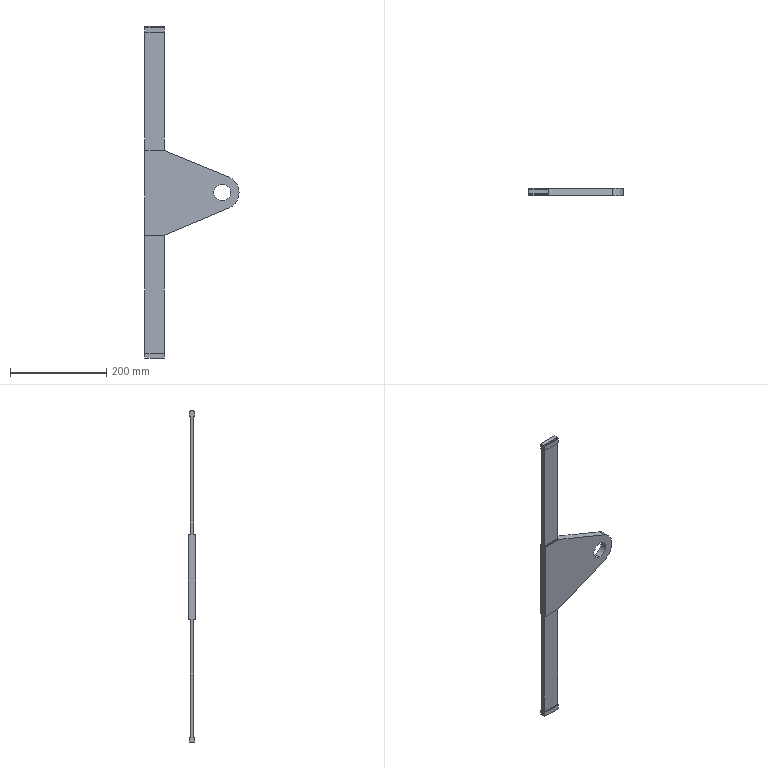Part | SolidWorks | features ICE 6, Cut 1, Extrusion 1, Fillet 1, MirrorPattern 1 | 1 solid | 36 faces | box 195.363 x 15 x 689 mm | volume 515152 mm3 | plane 29 | cylinder 7 | commonest cylinder face diameters 2 x4 35 x2 70 x1
STEP:
#1=CARTESIAN_POINT('',(140.363,7.5,18.413));
#2=VERTEX_POINT('',#1);
#3=CARTESIAN_POINT('',(140.363,7.5,-16.587));
#4=VERTEX_POINT('',#3);
#5=CARTESIAN_POINT('',(140.363,7.5,0.9129));
#6=DIRECTION('',(0.,-1.,0.));
#7=DIRECTION('',(0.,0.,-1.));
#8=AXIS2_PLACEMENT_3D('',#5,#6,#7);
#9=CIRCLE('',#8,17.5);
#10=EDGE_CURVE('',#2,#4,#9,.T.);
#11=ORIENTED_EDGE('',*,*,#10,.F.);
#12=CARTESIAN_POINT('',(140.363,-7.5,18.413));
#13=VERTEX_POINT('',#12);
#14=CARTESIAN_POINT('',(140.363,7.5,18.413));
#15=DIRECTION('',(0.,-1.,0.));
#16=VECTOR('',#15,1000.);
#17=LINE('',#14,#16);
#18=EDGE_CURVE('',#2,#13,#17,.T.);
#19=ORIENTED_EDGE('',*,*,#18,.T.);
#20=CARTESIAN_POINT('',(140.363,-7.5,-16.587));
#21=VERTEX_POINT('',#20);
#22=CARTESIAN_POINT('',(140.363,-7.5,0.9129));
#23=DIRECTION('',(0.,-1.,0.));
#24=DIRECTION('',(0.,0.,-1.));
#25=AXIS2_PLACEMENT_3D('',#22,#23,#24);
#26=CIRCLE('',#25,17.5);
#27=EDGE_CURVE('',#13,#21,#26,.T.);
#28=ORIENTED_EDGE('',*,*,#27,.T.);
#29=CARTESIAN_POINT('',(140.363,7.5,-16.587));
#30=DIRECTION('',(0.,-1.,0.));
#31=VECTOR('',#30,1000.);
#32=LINE('',#29,#31);
#33=EDGE_CURVE('',#4,#21,#32,.T.);
#34=ORIENTED_EDGE('',*,*,#33,.F.);
#35=EDGE_LOOP('',(#11,#19,#28,#34));
#36=FACE_OUTER_BOUND('',#35,.T.);
#37=CARTESIAN_POINT('',(140.363,7.5,0.9129));
#38=DIRECTION('',(0.,-1.,0.));
#39=DIRECTION('',(0.,0.,-1.));
#40=AXIS2_PLACEMENT_3D('',#37,#38,#39);
#41=CYLINDRICAL_SURFACE('',#40,17.5);
#42=ADVANCED_FACE('',(#36),#41,.F.);
#43=CARTESIAN_POINT('',(20.,-4.,-89.));
#44=VERTEX_POINT('',#43);
#45=CARTESIAN_POINT('',(20.,-4.,-332.5));
#46=VERTEX_POINT('',#45);
#47=CARTESIAN_POINT('',(20.,-4.,330.5));
#48=DIRECTION('',(0.,0.,-1.));
#49=VECTOR('',#48,1000.);
#50=LINE('',#47,#49);
#51=EDGE_CURVE('',#44,#46,#50,.T.);
#52=ORIENTED_EDGE('',*,*,#51,.T.);
#53=CARTESIAN_POINT('',(20.,-6.,-332.5));
#54=VERTEX_POINT('',#53);
#55=CARTESIAN_POINT('',(20.,4.,-332.5));
#56=DIRECTION('',(0.,-1.,0.));
#57=VECTOR('',#56,1000.);
#58=LINE('',#55,#57);
#59=EDGE_CURVE('',#46,#54,#58,.T.);
#60=ORIENTED_EDGE('',*,*,#59,.T.);
#61=CARTESIAN_POINT('',(20.,-6.,-342.5));
#62=VERTEX_POINT('',#61);
#63=CARTESIAN_POINT('',(20.,-6.,-333.5));
#64=DIRECTION('',(0.,0.,1.));
#65=VECTOR('',#64,1000.);
#66=LINE('',#63,#65);
#67=EDGE_CURVE('',#62,#54,#66,.T.);
#68=ORIENTED_EDGE('',*,*,#67,.F.);
#69=CARTESIAN_POINT('',(20.,6.,-342.5));
#70=VERTEX_POINT('',#69);
#71=CARTESIAN_POINT('',(20.,-4.,-342.5));
#72=DIRECTION('',(0.,-1.,0.));
#73=VECTOR('',#72,1000.);
#74=LINE('',#71,#73);
#75=EDGE_CURVE('',#70,#62,#74,.T.);
#76=ORIENTED_EDGE('',*,*,#75,.F.);
#77=CARTESIAN_POINT('',(20.,6.,-332.5));
#78=VERTEX_POINT('',#77);
#79=CARTESIAN_POINT('',(20.,6.,-333.5));
#80=DIRECTION('',(0.,0.,-1.));
#81=VECTOR('',#80,1000.);
#82=LINE('',#79,#81);
#83=EDGE_CURVE('',#78,#70,#82,.T.);
#84=ORIENTED_EDGE('',*,*,#83,.F.);
#85=CARTESIAN_POINT('',(20.,4.,-332.5));
#86=VERTEX_POINT('',#85);
#87=CARTESIAN_POINT('',(20.,4.,-332.5));
#88=DIRECTION('',(0.,-1.,0.));
#89=VECTOR('',#88,1000.);
#90=LINE('',#87,#89);
#91=EDGE_CURVE('',#78,#86,#90,.T.);
#92=ORIENTED_EDGE('',*,*,#91,.T.);
#93=CARTESIAN_POINT('',(20.,4.,-89.));
#94=VERTEX_POINT('',#93);
#95=CARTESIAN_POINT('',(20.,4.,330.5));
#96=DIRECTION('',(0.,0.,-1.));
#97=VECTOR('',#96,1000.);
#98=LINE('',#95,#97);
#99=EDGE_CURVE('',#94,#86,#98,.T.);
#100=ORIENTED_EDGE('',*,*,#99,.F.);
#101=CARTESIAN_POINT('',(20.,5.,-88.));
#102=VERTEX_POINT('',#101);
#103=CARTESIAN_POINT('',(20.,5.,-89.));
#104=DIRECTION('',(-1.,0.,0.));
#105=DIRECTION('',(0.,0.,1.));
#106=AXIS2_PLACEMENT_3D('',#103,#104,#105);
#107=CIRCLE('',#106,1.);
#108=EDGE_CURVE('',#94,#102,#107,.T.);
#109=ORIENTED_EDGE('',*,*,#108,.T.);
#110=CARTESIAN_POINT('',(20.,-5.,-88.));
#111=VERTEX_POINT('',#110);
#112=CARTESIAN_POINT('',(20.,-7.5,-88.));
#113=DIRECTION('',(0.,1.,0.));
#114=VECTOR('',#113,1000.);
#115=LINE('',#112,#114);
#116=EDGE_CURVE('',#111,#102,#115,.T.);
#117=ORIENTED_EDGE('',*,*,#116,.F.);
#118=CARTESIAN_POINT('',(20.,-5.,-89.));
#119=DIRECTION('',(-1.,0.,0.));
#120=DIRECTION('',(0.,0.,1.));
#121=AXIS2_PLACEMENT_3D('',#118,#119,#120);
#122=CIRCLE('',#121,1.);
#123=EDGE_CURVE('',#111,#44,#122,.T.);
#124=ORIENTED_EDGE('',*,*,#123,.T.);
#125=EDGE_LOOP('',(#52,#60,#68,#76,#84,#92,#100,#109,#117,#124));
#126=FACE_OUTER_BOUND('',#125,.T.);
#127=CARTESIAN_POINT('',(20.,-4.,330.5));
#128=DIRECTION('',(-1.,0.,0.));
#129=DIRECTION('',(0.,0.,1.));
#130=AXIS2_PLACEMENT_3D('',#127,#128,#129);
#131=PLANE('',#130);
#132=ADVANCED_FACE('',(#126),#131,.F.);
#133=CARTESIAN_POINT('',(-20.,4.,-89.));
#134=VERTEX_POINT('',#133);
#135=CARTESIAN_POINT('',(-20.,4.,-332.5));
#136=VERTEX_POINT('',#135);
#137=CARTESIAN_POINT('',(-20.,4.,330.5));
#138=DIRECTION('',(0.,0.,-1.));
#139=VECTOR('',#138,1000.);
#140=LINE('',#137,#139);
#141=EDGE_CURVE('',#134,#136,#140,.T.);
#142=ORIENTED_EDGE('',*,*,#141,.T.);
#143=CARTESIAN_POINT('',(-20.,6.,-332.5));
#144=VERTEX_POINT('',#143);
#145=CARTESIAN_POINT('',(-20.,4.,-332.5));
#146=DIRECTION('',(0.,1.,0.));
#147=VECTOR('',#146,1000.);
#148=LINE('',#145,#147);
#149=EDGE_CURVE('',#136,#144,#148,.T.);
#150=ORIENTED_EDGE('',*,*,#149,.T.);
#151=CARTESIAN_POINT('',(-20.,6.,-342.5));
#152=VERTEX_POINT('',#151);
#153=CARTESIAN_POINT('',(-20.,6.,-333.5));
#154=DIRECTION('',(0.,0.,1.));
#155=VECTOR('',#154,1000.);
#156=LINE('',#153,#155);
#157=EDGE_CURVE('',#152,#144,#156,.T.);
#158=ORIENTED_EDGE('',*,*,#157,.F.);
#159=CARTESIAN_POINT('',(-20.,-6.,-342.5));
#160=VERTEX_POINT('',#159);
#161=CARTESIAN_POINT('',(-20.,-4.,-342.5));
#162=DIRECTION('',(0.,1.,0.));
#163=VECTOR('',#162,1000.);
#164=LINE('',#161,#163);
#165=EDGE_CURVE('',#160,#152,#164,.T.);
#166=ORIENTED_EDGE('',*,*,#165,.F.);
#167=CARTESIAN_POINT('',(-20.,-6.,-332.5));
#168=VERTEX_POINT('',#167);
#169=CARTESIAN_POINT('',(-20.,-6.,-333.5));
#170=DIRECTION('',(0.,0.,-1.));
#171=VECTOR('',#170,1000.);
#172=LINE('',#169,#171);
#173=EDGE_CURVE('',#168,#160,#172,.T.);
#174=ORIENTED_EDGE('',*,*,#173,.F.);
#175=CARTESIAN_POINT('',(-20.,-4.,-332.5));
#176=VERTEX_POINT('',#175);
#177=CARTESIAN_POINT('',(-20.,4.,-332.5));
#178=DIRECTION('',(0.,1.,0.));
#179=VECTOR('',#178,1000.);
#180=LINE('',#177,#179);
#181=EDGE_CURVE('',#168,#176,#180,.T.);
#182=ORIENTED_EDGE('',*,*,#181,.T.);
#183=CARTESIAN_POINT('',(-20.,-4.,-89.));
#184=VERTEX_POINT('',#183);
#185=CARTESIAN_POINT('',(-20.,-4.,330.5));
#186=DIRECTION('',(0.,0.,-1.));
#187=VECTOR('',#186,1000.);
#188=LINE('',#185,#187);
#189=EDGE_CURVE('',#184,#176,#188,.T.);
#190=ORIENTED_EDGE('',*,*,#189,.F.);
#191=CARTESIAN_POINT('',(-20.,-5.,-88.));
#192=VERTEX_POINT('',#191);
#193=CARTESIAN_POINT('',(-20.,-5.,-89.));
#194=DIRECTION('',(1.,0.,0.));
#195=DIRECTION('',(0.,0.,-1.));
#196=AXIS2_PLACEMENT_3D('',#193,#194,#195);
#197=CIRCLE('',#196,1.);
#198=EDGE_CURVE('',#184,#192,#197,.T.);
#199=ORIENTED_EDGE('',*,*,#198,.T.);
#200=CARTESIAN_POINT('',(-20.,-7.5,-88.));
#201=VERTEX_POINT('',#200);
#202=CARTESIAN_POINT('',(-20.,-4.,-88.));
#203=DIRECTION('',(0.,1.,0.));
#204=VECTOR('',#203,1000.);
#205=LINE('',#202,#204);
#206=EDGE_CURVE('',#201,#192,#205,.T.);
#207=ORIENTED_EDGE('',*,*,#206,.F.);
#208=CARTESIAN_POINT('',(-20.,-7.5,88.));
#209=VERTEX_POINT('',#208);
#210=CARTESIAN_POINT('',(-20.,-7.5,-88.));
#211=DIRECTION('',(0.,0.,-1.));
#212=VECTOR('',#211,1000.);
#213=LINE('',#210,#212);
#214=EDGE_CURVE('',#209,#201,#213,.T.);
#215=ORIENTED_EDGE('',*,*,#214,.F.);
#216=CARTESIAN_POINT('',(-20.,-5.,88.));
#217=VERTEX_POINT('',#216);
#218=CARTESIAN_POINT('',(-20.,-7.5,88.));
#219=DIRECTION('',(0.,-1.,0.));
#220=VECTOR('',#219,1000.);
#221=LINE('',#218,#220);
#222=EDGE_CURVE('',#217,#209,#221,.T.);
#223=ORIENTED_EDGE('',*,*,#222,.F.);
#224=CARTESIAN_POINT('',(-20.,-4.,89.));
#225=VERTEX_POINT('',#224);
#226=CARTESIAN_POINT('',(-20.,-5.,89.));
#227=DIRECTION('',(1.,0.,0.));
#228=DIRECTION('',(0.,0.,-1.));
#229=AXIS2_PLACEMENT_3D('',#226,#227,#228);
#230=CIRCLE('',#229,1.);
#231=EDGE_CURVE('',#217,#225,#230,.T.);
#232=ORIENTED_EDGE('',*,*,#231,.T.);
#233=CARTESIAN_POINT('',(-20.,-4.,333.5));
#234=VERTEX_POINT('',#233);
#235=CARTESIAN_POINT('',(-20.,-4.,330.5));
#236=DIRECTION('',(0.,0.,-1.));
#237=VECTOR('',#236,1000.);
#238=LINE('',#235,#237);
#239=EDGE_CURVE('',#234,#225,#238,.T.);
#240=ORIENTED_EDGE('',*,*,#239,.F.);
#241=CARTESIAN_POINT('',(-20.,-6.,333.5));
#242=VERTEX_POINT('',#241);
#243=CARTESIAN_POINT('',(-20.,-6.,333.5));
#244=DIRECTION('',(0.,-1.,0.));
#245=VECTOR('',#244,1000.);
#246=LINE('',#243,#245);
#247=EDGE_CURVE('',#234,#242,#246,.T.);
#248=ORIENTED_EDGE('',*,*,#247,.T.);
#249=CARTESIAN_POINT('',(-20.,-6.,343.5));
#250=VERTEX_POINT('',#249);
#251=CARTESIAN_POINT('',(-20.,-6.,333.5));
#252=DIRECTION('',(0.,0.,1.));
#253=VECTOR('',#252,1000.);
#254=LINE('',#251,#253);
#255=EDGE_CURVE('',#242,#250,#254,.T.);
#256=ORIENTED_EDGE('',*,*,#255,.T.);
#257=CARTESIAN_POINT('',(-20.,-4.,343.5));
#258=VERTEX_POINT('',#257);
#259=CARTESIAN_POINT('',(-20.,-6.,343.5));
#260=DIRECTION('',(0.,1.,0.));
#261=VECTOR('',#260,1000.);
#262=LINE('',#259,#261);
#263=EDGE_CURVE('',#250,#258,#262,.T.);
#264=ORIENTED_EDGE('',*,*,#263,.T.);
#265=CARTESIAN_POINT('',(-20.,-4.,346.5));
#266=VERTEX_POINT('',#265);
#267=CARTESIAN_POINT('',(-20.,-4.,343.5));
#268=DIRECTION('',(0.,0.,1.));
#269=VECTOR('',#268,1000.);
#270=LINE('',#267,#269);
#271=EDGE_CURVE('',#258,#266,#270,.T.);
#272=ORIENTED_EDGE('',*,*,#271,.T.);
#273=CARTESIAN_POINT('',(-20.,4.,346.5));
#274=VERTEX_POINT('',#273);
#275=CARTESIAN_POINT('',(-20.,0.5169,346.5));
#276=DIRECTION('',(0.,1.,0.));
#277=VECTOR('',#276,1000.);
#278=LINE('',#275,#277);
#279=EDGE_CURVE('',#266,#274,#278,.T.);
#280=ORIENTED_EDGE('',*,*,#279,.T.);
#281=CARTESIAN_POINT('',(-20.,4.,343.5));
#282=VERTEX_POINT('',#281);
#283=CARTESIAN_POINT('',(-20.,4.,343.5));
#284=DIRECTION('',(0.,0.,-1.));
#285=VECTOR('',#284,1000.);
#286=LINE('',#283,#285);
#287=EDGE_CURVE('',#274,#282,#286,.T.);
#288=ORIENTED_EDGE('',*,*,#287,.T.);
#289=CARTESIAN_POINT('',(-20.,6.,343.5));
#290=VERTEX_POINT('',#289);
#291=CARTESIAN_POINT('',(-20.,4.,343.5));
#292=DIRECTION('',(0.,1.,0.));
#293=VECTOR('',#292,1000.);
#294=LINE('',#291,#293);
#295=EDGE_CURVE('',#282,#290,#294,.T.);
#296=ORIENTED_EDGE('',*,*,#295,.T.);
#297=CARTESIAN_POINT('',(-20.,6.,333.5));
#298=VERTEX_POINT('',#297);
#299=CARTESIAN_POINT('',(-20.,6.,333.5));
#300=DIRECTION('',(0.,0.,-1.));
#301=VECTOR('',#300,1000.);
#302=LINE('',#299,#301);
#303=EDGE_CURVE('',#290,#298,#302,.T.);
#304=ORIENTED_EDGE('',*,*,#303,.T.);
#305=CARTESIAN_POINT('',(-20.,4.,333.5));
#306=VERTEX_POINT('',#305);
#307=CARTESIAN_POINT('',(-20.,4.,333.5));
#308=DIRECTION('',(0.,-1.,0.));
#309=VECTOR('',#308,1000.);
#310=LINE('',#307,#309);
#311=EDGE_CURVE('',#298,#306,#310,.T.);
#312=ORIENTED_EDGE('',*,*,#311,.T.);
#313=CARTESIAN_POINT('',(-20.,4.,89.));
#314=VERTEX_POINT('',#313);
#315=CARTESIAN_POINT('',(-20.,4.,330.5));
#316=DIRECTION('',(0.,0.,-1.));
#317=VECTOR('',#316,1000.);
#318=LINE('',#315,#317);
#319=EDGE_CURVE('',#306,#314,#318,.T.);
#320=ORIENTED_EDGE('',*,*,#319,.T.);
#321=CARTESIAN_POINT('',(-20.,5.,88.));
#322=VERTEX_POINT('',#321);
#323=CARTESIAN_POINT('',(-20.,5.,89.));
#324=DIRECTION('',(1.,0.,0.));
#325=DIRECTION('',(0.,0.,-1.));
#326=AXIS2_PLACEMENT_3D('',#323,#324,#325);
#327=CIRCLE('',#326,1.);
#328=EDGE_CURVE('',#314,#322,#327,.T.);
#329=ORIENTED_EDGE('',*,*,#328,.T.);
#330=CARTESIAN_POINT('',(-20.,7.5,88.));
#331=VERTEX_POINT('',#330);
#332=CARTESIAN_POINT('',(-20.,4.,88.));
#333=DIRECTION('',(0.,-1.,0.));
#334=VECTOR('',#333,1000.);
#335=LINE('',#332,#334);
#336=EDGE_CURVE('',#331,#322,#335,.T.);
#337=ORIENTED_EDGE('',*,*,#336,.F.);
#338=CARTESIAN_POINT('',(-20.,7.5,-88.));
#339=VERTEX_POINT('',#338);
#340=CARTESIAN_POINT('',(-20.,7.5,88.));
#341=DIRECTION('',(0.,0.,1.));
#342=VECTOR('',#341,1000.);
#343=LINE('',#340,#342);
#344=EDGE_CURVE('',#339,#331,#343,.T.);
#345=ORIENTED_EDGE('',*,*,#344,.F.);
#346=CARTESIAN_POINT('',(-20.,5.,-88.));
#347=VERTEX_POINT('',#346);
#348=CARTESIAN_POINT('',(-20.,7.5,-88.));
#349=DIRECTION('',(0.,1.,0.));
#350=VECTOR('',#349,1000.);
#351=LINE('',#348,#350);
#352=EDGE_CURVE('',#347,#339,#351,.T.);
#353=ORIENTED_EDGE('',*,*,#352,.F.);
#354=CARTESIAN_POINT('',(-20.,5.,-89.));
#355=DIRECTION('',(1.,0.,0.));
#356=DIRECTION('',(0.,0.,-1.));
#357=AXIS2_PLACEMENT_3D('',#354,#355,#356);
#358=CIRCLE('',#357,1.);
#359=EDGE_CURVE('',#347,#134,#358,.T.);
#360=ORIENTED_EDGE('',*,*,#359,.T.);
#361=EDGE_LOOP('',(#142,#150,#158,#166,#174,#182,#190,#199,#207,#215,#223,#232,#240,#248,#256,#264,#272,#280,#288,#296,#304,#312,#320,#329,#337,#345,#353,#360));
#362=FACE_OUTER_BOUND('',#361,.T.);
#363=CARTESIAN_POINT('',(-20.,-4.,330.5));
#364=DIRECTION('',(1.,0.,0.));
#365=DIRECTION('',(0.,0.,-1.));
#366=AXIS2_PLACEMENT_3D('',#363,#364,#365);
#367=PLANE('',#366);
#368=ADVANCED_FACE('',(#362),#367,.F.);
#369=ORIENTED_EDGE('',*,*,#83,.T.);
#370=CARTESIAN_POINT('',(35.62,6.,-342.5));
#371=DIRECTION('',(-1.,0.,0.));
#372=VECTOR('',#371,1000.);
#373=LINE('',#370,#372);
#374=EDGE_CURVE('',#70,#152,#373,.T.);
#375=ORIENTED_EDGE('',*,*,#374,.T.);
#376=ORIENTED_EDGE('',*,*,#157,.T.);
#377=CARTESIAN_POINT('',(35.62,6.,-332.5));
#378=DIRECTION('',(-1.,0.,0.));
#379=VECTOR('',#378,1000.);
#380=LINE('',#377,#379);
#381=EDGE_CURVE('',#78,#144,#380,.T.);
#382=ORIENTED_EDGE('',*,*,#381,.F.);
#383=EDGE_LOOP('',(#369,#375,#376,#382));
#384=FACE_OUTER_BOUND('',#383,.T.);
#385=CARTESIAN_POINT('',(40.,6.,-333.5));
#386=DIRECTION('',(0.,-1.,0.));
#387=DIRECTION('',(0.,0.,-1.));
#388=AXIS2_PLACEMENT_3D('',#385,#386,#387);
#389=PLANE('',#388);
#390=ADVANCED_FACE('',(#384),#389,.F.);
#391=ORIENTED_EDGE('',*,*,#173,.T.);
#392=CARTESIAN_POINT('',(35.62,-6.,-342.5));
#393=DIRECTION('',(-1.,0.,0.));
#394=VECTOR('',#393,1000.);
#395=LINE('',#392,#394);
#396=EDGE_CURVE('',#62,#160,#395,.T.);
#397=ORIENTED_EDGE('',*,*,#396,.F.);
#398=ORIENTED_EDGE('',*,*,#67,.T.);
#399=CARTESIAN_POINT('',(35.62,-6.,-332.5));
#400=DIRECTION('',(-1.,0.,0.));
#401=VECTOR('',#400,1000.);
#402=LINE('',#399,#401);
#403=EDGE_CURVE('',#54,#168,#402,.T.);
#404=ORIENTED_EDGE('',*,*,#403,.T.);
#405=EDGE_LOOP('',(#391,#397,#398,#404));
#406=FACE_OUTER_BOUND('',#405,.T.);
#407=CARTESIAN_POINT('',(40.,-6.,-333.5));
#408=DIRECTION('',(0.,1.,0.));
#409=DIRECTION('',(0.,0.,1.));
#410=AXIS2_PLACEMENT_3D('',#407,#408,#409);
#411=PLANE('',#410);
#412=ADVANCED_FACE('',(#406),#411,.F.);
#413=ORIENTED_EDGE('',*,*,#189,.T.);
#414=CARTESIAN_POINT('',(-20.,-4.,-332.5));
#415=DIRECTION('',(1.,0.,0.));
#416=VECTOR('',#415,1000.);
#417=LINE('',#414,#416);
#418=EDGE_CURVE('',#176,#46,#417,.T.);
#419=ORIENTED_EDGE('',*,*,#418,.T.);
#420=ORIENTED_EDGE('',*,*,#51,.F.);
#421=CARTESIAN_POINT('',(-20.,-4.,-89.));
#422=DIRECTION('',(-1.,0.,0.));
#423=VECTOR('',#422,1000.);
#424=LINE('',#421,#423);
#425=EDGE_CURVE('',#44,#184,#424,.T.);
#426=ORIENTED_EDGE('',*,*,#425,.T.);
#427=EDGE_LOOP('',(#413,#419,#420,#426));
#428=FACE_OUTER_BOUND('',#427,.T.);
#429=CARTESIAN_POINT('',(-20.,-4.,330.5));
#430=DIRECTION('',(0.,1.,0.));
#431=DIRECTION('',(0.,0.,1.));
#432=AXIS2_PLACEMENT_3D('',#429,#430,#431);
#433=PLANE('',#432);
#434=ADVANCED_FACE('',(#428),#433,.F.);
#435=ORIENTED_EDGE('',*,*,#239,.T.);
#436=CARTESIAN_POINT('',(20.,-4.,89.));
#437=VERTEX_POINT('',#436);
#438=CARTESIAN_POINT('',(20.,-4.,89.));
#439=DIRECTION('',(1.,0.,0.));
#440=VECTOR('',#439,1000.);
#441=LINE('',#438,#440);
#442=EDGE_CURVE('',#225,#437,#441,.T.);
#443=ORIENTED_EDGE('',*,*,#442,.T.);
#444=CARTESIAN_POINT('',(20.,-4.,333.5));
#445=VERTEX_POINT('',#444);
#446=CARTESIAN_POINT('',(20.,-4.,330.5));
#447=DIRECTION('',(0.,0.,-1.));
#448=VECTOR('',#447,1000.);
#449=LINE('',#446,#448);
#450=EDGE_CURVE('',#445,#437,#449,.T.);
#451=ORIENTED_EDGE('',*,*,#450,.F.);
#452=CARTESIAN_POINT('',(40.,-4.,333.5));
#453=DIRECTION('',(-1.,0.,0.));
#454=VECTOR('',#453,1000.);
#455=LINE('',#452,#454);
#456=EDGE_CURVE('',#445,#234,#455,.T.);
#457=ORIENTED_EDGE('',*,*,#456,.T.);
#458=EDGE_LOOP('',(#435,#443,#451,#457));
#459=FACE_OUTER_BOUND('',#458,.T.);
#460=CARTESIAN_POINT('',(-20.,-4.,330.5));
#461=DIRECTION('',(0.,1.,0.));
#462=DIRECTION('',(0.,0.,1.));
#463=AXIS2_PLACEMENT_3D('',#460,#461,#462);
#464=PLANE('',#463);
#465=ADVANCED_FACE('',(#459),#464,.F.);
#466=CARTESIAN_POINT('',(20.,4.,333.5));
#467=VERTEX_POINT('',#466);
#468=CARTESIAN_POINT('',(20.,4.,89.));
#469=VERTEX_POINT('',#468);
#470=CARTESIAN_POINT('',(20.,4.,330.5));
#471=DIRECTION('',(0.,0.,-1.));
#472=VECTOR('',#471,1000.);
#473=LINE('',#470,#472);
#474=EDGE_CURVE('',#467,#469,#473,.T.);
#475=ORIENTED_EDGE('',*,*,#474,.T.);
#476=CARTESIAN_POINT('',(-20.,4.,89.));
#477=DIRECTION('',(-1.,0.,0.));
#478=VECTOR('',#477,1000.);
#479=LINE('',#476,#478);
#480=EDGE_CURVE('',#469,#314,#479,.T.);
#481=ORIENTED_EDGE('',*,*,#480,.T.);
#482=ORIENTED_EDGE('',*,*,#319,.F.);
#483=CARTESIAN_POINT('',(40.,4.,333.5));
#484=DIRECTION('',(-1.,0.,0.));
#485=VECTOR('',#484,1000.);
#486=LINE('',#483,#485);
#487=EDGE_CURVE('',#467,#306,#486,.T.);
#488=ORIENTED_EDGE('',*,*,#487,.F.);
#489=EDGE_LOOP('',(#475,#481,#482,#488));
#490=FACE_OUTER_BOUND('',#489,.T.);
#491=CARTESIAN_POINT('',(-20.,4.,330.5));
#492=DIRECTION('',(0.,-1.,0.));
#493=DIRECTION('',(0.,0.,-1.));
#494=AXIS2_PLACEMENT_3D('',#491,#492,#493);
#495=PLANE('',#494);
#496=ADVANCED_FACE('',(#490),#495,.F.);
#497=ORIENTED_EDGE('',*,*,#99,.T.);
#498=CARTESIAN_POINT('',(-20.,4.,-332.5));
#499=DIRECTION('',(-1.,0.,0.));
#500=VECTOR('',#499,1000.);
#501=LINE('',#498,#500);
#502=EDGE_CURVE('',#86,#136,#501,.T.);
#503=ORIENTED_EDGE('',*,*,#502,.T.);
#504=ORIENTED_EDGE('',*,*,#141,.F.);
#505=CARTESIAN_POINT('',(20.,4.,-89.));
#506=DIRECTION('',(1.,0.,0.));
#507=VECTOR('',#506,1000.);
#508=LINE('',#505,#507);
#509=EDGE_CURVE('',#134,#94,#508,.T.);
#510=ORIENTED_EDGE('',*,*,#509,.T.);
#511=EDGE_LOOP('',(#497,#503,#504,#510));
#512=FACE_OUTER_BOUND('',#511,.T.);
#513=CARTESIAN_POINT('',(-20.,4.,330.5));
#514=DIRECTION('',(0.,-1.,0.));
#515=DIRECTION('',(0.,0.,-1.));
#516=AXIS2_PLACEMENT_3D('',#513,#514,#515);
#517=PLANE('',#516);
#518=ADVANCED_FACE('',(#512),#517,.F.);
#519=ORIENTED_EDGE('',*,*,#450,.T.);
#520=CARTESIAN_POINT('',(20.,-5.,88.));
#521=VERTEX_POINT('',#520);
#522=CARTESIAN_POINT('',(20.,-5.,89.));
#523=DIRECTION('',(-1.,0.,0.));
#524=DIRECTION('',(0.,0.,1.));
#525=AXIS2_PLACEMENT_3D('',#522,#523,#524);
#526=CIRCLE('',#525,1.);
#527=EDGE_CURVE('',#437,#521,#526,.T.);
#528=ORIENTED_EDGE('',*,*,#527,.T.);
#529=CARTESIAN_POINT('',(20.,5.,88.));
#530=VERTEX_POINT('',#529);
#531=CARTESIAN_POINT('',(20.,-7.5,88.));
#532=DIRECTION('',(0.,1.,0.));
#533=VECTOR('',#532,1000.);
#534=LINE('',#531,#533);
#535=EDGE_CURVE('',#521,#530,#534,.T.);
#536=ORIENTED_EDGE('',*,*,#535,.T.);
#537=CARTESIAN_POINT('',(20.,5.,89.));
#538=DIRECTION('',(-1.,0.,0.));
#539=DIRECTION('',(0.,0.,1.));
#540=AXIS2_PLACEMENT_3D('',#537,#538,#539);
#541=CIRCLE('',#540,1.);
#542=EDGE_CURVE('',#530,#469,#541,.T.);
#543=ORIENTED_EDGE('',*,*,#542,.T.);
#544=ORIENTED_EDGE('',*,*,#474,.F.);
#545=CARTESIAN_POINT('',(20.,6.,333.5));
#546=VERTEX_POINT('',#545);
#547=CARTESIAN_POINT('',(20.,4.,333.5));
#548=DIRECTION('',(0.,1.,0.));
#549=VECTOR('',#548,1000.);
#550=LINE('',#547,#549);
#551=EDGE_CURVE('',#467,#546,#550,.T.);
#552=ORIENTED_EDGE('',*,*,#551,.T.);
#553=CARTESIAN_POINT('',(20.,6.,343.5));
#554=VERTEX_POINT('',#553);
#555=CARTESIAN_POINT('',(20.,6.,333.5));
#556=DIRECTION('',(0.,0.,1.));
#557=VECTOR('',#556,1000.);
#558=LINE('',#555,#557);
#559=EDGE_CURVE('',#546,#554,#558,.T.);
#560=ORIENTED_EDGE('',*,*,#559,.T.);
#561=CARTESIAN_POINT('',(20.,4.,343.5));
#562=VERTEX_POINT('',#561);
#563=CARTESIAN_POINT('',(20.,4.,343.5));
#564=DIRECTION('',(0.,-1.,0.));
#565=VECTOR('',#564,1000.);
#566=LINE('',#563,#565);
#567=EDGE_CURVE('',#554,#562,#566,.T.);
#568=ORIENTED_EDGE('',*,*,#567,.T.);
#569=CARTESIAN_POINT('',(20.,4.,346.5));
#570=VERTEX_POINT('',#569);
#571=CARTESIAN_POINT('',(20.,4.,343.5));
#572=DIRECTION('',(0.,0.,1.));
#573=VECTOR('',#572,1000.);
#574=LINE('',#571,#573);
#575=EDGE_CURVE('',#562,#570,#574,.T.);
#576=ORIENTED_EDGE('',*,*,#575,.T.);
#577=CARTESIAN_POINT('',(20.,-4.,346.5));
#578=VERTEX_POINT('',#577);
#579=CARTESIAN_POINT('',(20.,0.5169,346.5));
#580=DIRECTION('',(0.,-1.,0.));
#581=VECTOR('',#580,1000.);
#582=LINE('',#579,#581);
#583=EDGE_CURVE('',#570,#578,#582,.T.);
#584=ORIENTED_EDGE('',*,*,#583,.T.);
#585=CARTESIAN_POINT('',(20.,-4.,343.5));
#586=VERTEX_POINT('',#585);
#587=CARTESIAN_POINT('',(20.,-4.,343.5));
#588=DIRECTION('',(0.,0.,-1.));
#589=VECTOR('',#588,1000.);
#590=LINE('',#587,#589);
#591=EDGE_CURVE('',#578,#586,#590,.T.);
#592=ORIENTED_EDGE('',*,*,#591,.T.);
#593=CARTESIAN_POINT('',(20.,-6.,343.5));
#594=VERTEX_POINT('',#593);
#595=CARTESIAN_POINT('',(20.,-6.,343.5));
#596=DIRECTION('',(0.,-1.,0.));
#597=VECTOR('',#596,1000.);
#598=LINE('',#595,#597);
#599=EDGE_CURVE('',#586,#594,#598,.T.);
#600=ORIENTED_EDGE('',*,*,#599,.T.);
#601=CARTESIAN_POINT('',(20.,-6.,333.5));
#602=VERTEX_POINT('',#601);
#603=CARTESIAN_POINT('',(20.,-6.,333.5));
#604=DIRECTION('',(0.,0.,-1.));
#605=VECTOR('',#604,1000.);
#606=LINE('',#603,#605);
#607=EDGE_CURVE('',#594,#602,#606,.T.);
#608=ORIENTED_EDGE('',*,*,#607,.T.);
#609=CARTESIAN_POINT('',(20.,-6.,333.5));
#610=DIRECTION('',(0.,1.,0.));
#611=VECTOR('',#610,1000.);
#612=LINE('',#609,#611);
#613=EDGE_CURVE('',#602,#445,#612,.T.);
#614=ORIENTED_EDGE('',*,*,#613,.T.);
#615=EDGE_LOOP('',(#519,#528,#536,#543,#544,#552,#560,#568,#576,#584,#592,#600,#608,#614));
#616=FACE_OUTER_BOUND('',#615,.T.);
#617=CARTESIAN_POINT('',(20.,-4.,330.5));
#618=DIRECTION('',(-1.,0.,0.));
#619=DIRECTION('',(0.,0.,1.));
#620=AXIS2_PLACEMENT_3D('',#617,#618,#619);
#621=PLANE('',#620);
#622=ADVANCED_FACE('',(#616),#621,.F.);
#623=CARTESIAN_POINT('',(20.,7.5,-88.));
#624=VERTEX_POINT('',#623);
#625=CARTESIAN_POINT('',(153.998,7.5,-31.322));
#626=VERTEX_POINT('',#625);
#627=CARTESIAN_POINT('',(153.998,7.5,-31.322));
#628=DIRECTION('',(0.921,0.,0.3896));
#629=VECTOR('',#628,1000.);
#630=LINE('',#627,#629);
#631=EDGE_CURVE('',#624,#626,#630,.T.);
#632=ORIENTED_EDGE('',*,*,#631,.T.);
#633=CARTESIAN_POINT('',(153.998,-7.5,-31.322));
#634=VERTEX_POINT('',#633);
#635=CARTESIAN_POINT('',(153.998,-7.5,-31.322));
#636=DIRECTION('',(0.,1.,0.));
#637=VECTOR('',#636,1000.);
#638=LINE('',#635,#637);
#639=EDGE_CURVE('',#634,#626,#638,.T.);
#640=ORIENTED_EDGE('',*,*,#639,.F.);
#641=CARTESIAN_POINT('',(20.,-7.5,-88.));
#642=VERTEX_POINT('',#641);
#643=CARTESIAN_POINT('',(153.998,-7.5,-31.322));
#644=DIRECTION('',(0.921,0.,0.3896));
#645=VECTOR('',#644,1000.);
#646=LINE('',#643,#645);
#647=EDGE_CURVE('',#642,#634,#646,.T.);
#648=ORIENTED_EDGE('',*,*,#647,.F.);
#649=CARTESIAN_POINT('',(20.,-7.5,-88.));
#650=DIRECTION('',(0.,1.,0.));
#651=VECTOR('',#650,1000.);
#652=LINE('',#649,#651);
#653=EDGE_CURVE('',#642,#111,#652,.T.);
#654=ORIENTED_EDGE('',*,*,#653,.T.);
#655=ORIENTED_EDGE('',*,*,#116,.T.);
#656=CARTESIAN_POINT('',(20.,-7.5,-88.));
#657=DIRECTION('',(0.,1.,0.));
#658=VECTOR('',#657,1000.);
#659=LINE('',#656,#658);
#660=EDGE_CURVE('',#102,#624,#659,.T.);
#661=ORIENTED_EDGE('',*,*,#660,.T.);
#662=EDGE_LOOP('',(#632,#640,#648,#654,#655,#661));
#663=FACE_OUTER_BOUND('',#662,.T.);
#664=CARTESIAN_POINT('',(153.998,-7.5,-31.322));
#665=DIRECTION('',(-0.3896,0.,0.921));
#666=DIRECTION('',(0.921,0.,0.3896));
#667=AXIS2_PLACEMENT_3D('',#664,#665,#666);
#668=PLANE('',#667);
#669=ADVANCED_FACE('',(#663),#668,.F.);
#670=CARTESIAN_POINT('',(153.622,7.5,33.304));
#671=VERTEX_POINT('',#670);
#672=CARTESIAN_POINT('',(140.363,7.5,0.9129));
#673=DIRECTION('',(0.,-1.,0.));
#674=DIRECTION('',(0.,0.,-1.));
#675=AXIS2_PLACEMENT_3D('',#672,#673,#674);
#676=CIRCLE('',#675,35.);
#677=EDGE_CURVE('',#626,#671,#676,.T.);
#678=ORIENTED_EDGE('',*,*,#677,.T.);
#679=CARTESIAN_POINT('',(153.622,-7.5,33.304));
#680=VERTEX_POINT('',#679);
#681=CARTESIAN_POINT('',(153.622,-7.5,33.304));
#682=DIRECTION('',(0.,1.,0.));
#683=VECTOR('',#682,1000.);
#684=LINE('',#681,#683);
#685=EDGE_CURVE('',#680,#671,#684,.T.);
#686=ORIENTED_EDGE('',*,*,#685,.F.);
#687=CARTESIAN_POINT('',(140.363,-7.5,0.9129));
#688=DIRECTION('',(0.,-1.,0.));
#689=DIRECTION('',(0.,0.,-1.));
#690=AXIS2_PLACEMENT_3D('',#687,#688,#689);
#691=CIRCLE('',#690,35.);
#692=EDGE_CURVE('',#634,#680,#691,.T.);
#693=ORIENTED_EDGE('',*,*,#692,.F.);
#694=ORIENTED_EDGE('',*,*,#639,.T.);
#695=EDGE_LOOP('',(#678,#686,#693,#694));
#696=FACE_OUTER_BOUND('',#695,.T.);
#697=CARTESIAN_POINT('',(140.363,-7.5,0.9129));
#698=DIRECTION('',(0.,1.,0.));
#699=DIRECTION('',(0.,0.,1.));
#700=AXIS2_PLACEMENT_3D('',#697,#698,#699);
#701=CYLINDRICAL_SURFACE('',#700,35.);
#702=ADVANCED_FACE('',(#696),#701,.T.);
#703=CARTESIAN_POINT('',(20.,7.5,88.));
#704=VERTEX_POINT('',#703);
#705=CARTESIAN_POINT('',(153.622,7.5,33.304));
#706=DIRECTION('',(-0.9255,0.,0.3788));
#707=VECTOR('',#706,1000.);
#708=LINE('',#705,#707);
#709=EDGE_CURVE('',#671,#704,#708,.T.);
#710=ORIENTED_EDGE('',*,*,#709,.T.);
#711=CARTESIAN_POINT('',(20.,-7.5,88.));
#712=DIRECTION('',(0.,1.,0.));
#713=VECTOR('',#712,1000.);
#714=LINE('',#711,#713);
#715=EDGE_CURVE('',#530,#704,#714,.T.);
#716=ORIENTED_EDGE('',*,*,#715,.F.);
#717=ORIENTED_EDGE('',*,*,#535,.F.);
#718=CARTESIAN_POINT('',(20.,-7.5,88.));
#719=VERTEX_POINT('',#718);
#720=CARTESIAN_POINT('',(20.,-7.5,88.));
#721=DIRECTION('',(0.,1.,0.));
#722=VECTOR('',#721,1000.);
#723=LINE('',#720,#722);
#724=EDGE_CURVE('',#719,#521,#723,.T.);
#725=ORIENTED_EDGE('',*,*,#724,.F.);
#726=CARTESIAN_POINT('',(153.622,-7.5,33.304));
#727=DIRECTION('',(-0.9255,0.,0.3788));
#728=VECTOR('',#727,1000.);
#729=LINE('',#726,#728);
#730=EDGE_CURVE('',#680,#719,#729,.T.);
#731=ORIENTED_EDGE('',*,*,#730,.F.);
#732=ORIENTED_EDGE('',*,*,#685,.T.);
#733=EDGE_LOOP('',(#710,#716,#717,#725,#731,#732));
#734=FACE_OUTER_BOUND('',#733,.T.);
#735=CARTESIAN_POINT('',(153.622,-7.5,33.304));
#736=DIRECTION('',(-0.3788,0.,-0.9255));
#737=DIRECTION('',(-0.9255,0.,0.3788));
#738=AXIS2_PLACEMENT_3D('',#735,#736,#737);
#739=PLANE('',#738);
#740=ADVANCED_FACE('',(#734),#739,.F.);
#741=CARTESIAN_POINT('',(140.363,-7.5,0.9129));
#742=DIRECTION('',(0.,-1.,0.));
#743=DIRECTION('',(0.,0.,-1.));
#744=AXIS2_PLACEMENT_3D('',#741,#742,#743);
#745=CIRCLE('',#744,17.5);
#746=EDGE_CURVE('',#21,#13,#745,.T.);
#747=ORIENTED_EDGE('',*,*,#746,.F.);
#748=ORIENTED_EDGE('',*,*,#27,.F.);
#749=EDGE_LOOP('',(#747,#748));
#750=FACE_BOUND('',#749,.T.);
#751=ORIENTED_EDGE('',*,*,#730,.T.);
#752=CARTESIAN_POINT('',(-196.035,-7.5,88.));
#753=DIRECTION('',(1.,0.,0.));
#754=VECTOR('',#753,1000.);
#755=LINE('',#752,#754);
#756=EDGE_CURVE('',#209,#719,#755,.T.);
#757=ORIENTED_EDGE('',*,*,#756,.F.);
#758=ORIENTED_EDGE('',*,*,#214,.T.);
#759=CARTESIAN_POINT('',(-196.035,-7.5,-88.));
#760=DIRECTION('',(1.,0.,0.));
#761=VECTOR('',#760,1000.);
#762=LINE('',#759,#761);
#763=EDGE_CURVE('',#201,#642,#762,.T.);
#764=ORIENTED_EDGE('',*,*,#763,.T.);
#765=ORIENTED_EDGE('',*,*,#647,.T.);
#766=ORIENTED_EDGE('',*,*,#692,.T.);
#767=EDGE_LOOP('',(#751,#757,#758,#764,#765,#766));
#768=FACE_OUTER_BOUND('',#767,.T.);
#769=CARTESIAN_POINT('',(140.363,-7.5,0.9129));
#770=DIRECTION('',(0.,-1.,0.));
#771=DIRECTION('',(0.,0.,-1.));
#772=AXIS2_PLACEMENT_3D('',#769,#770,#771);
#773=PLANE('',#772);
#774=ADVANCED_FACE('',(#750,#768),#773,.T.);
#775=CARTESIAN_POINT('',(140.363,7.5,0.9129));
#776=DIRECTION('',(0.,-1.,0.));
#777=DIRECTION('',(0.,0.,-1.));
#778=AXIS2_PLACEMENT_3D('',#775,#776,#777);
#779=CIRCLE('',#778,17.5);
#780=EDGE_CURVE('',#4,#2,#779,.T.);
#781=ORIENTED_EDGE('',*,*,#780,.T.);
#782=ORIENTED_EDGE('',*,*,#10,.T.);
#783=EDGE_LOOP('',(#781,#782));
#784=FACE_BOUND('',#783,.T.);
#785=ORIENTED_EDGE('',*,*,#631,.F.);
#786=CARTESIAN_POINT('',(-196.035,7.5,-88.));
#787=DIRECTION('',(1.,0.,0.));
#788=VECTOR('',#787,1000.);
#789=LINE('',#786,#788);
#790=EDGE_CURVE('',#339,#624,#789,.T.);
#791=ORIENTED_EDGE('',*,*,#790,.F.);
#792=ORIENTED_EDGE('',*,*,#344,.T.);
#793=CARTESIAN_POINT('',(-196.035,7.5,88.));
#794=DIRECTION('',(1.,0.,0.));
#795=VECTOR('',#794,1000.);
#796=LINE('',#793,#795);
#797=EDGE_CURVE('',#331,#704,#796,.T.);
#798=ORIENTED_EDGE('',*,*,#797,.T.);
#799=ORIENTED_EDGE('',*,*,#709,.F.);
#800=ORIENTED_EDGE('',*,*,#677,.F.);
#801=EDGE_LOOP('',(#785,#791,#792,#798,#799,#800));
#802=FACE_OUTER_BOUND('',#801,.T.);
#803=CARTESIAN_POINT('',(140.363,7.5,0.9129));
#804=DIRECTION('',(0.,-1.,0.));
#805=DIRECTION('',(0.,0.,-1.));
#806=AXIS2_PLACEMENT_3D('',#803,#804,#805);
#807=PLANE('',#806);
#808=ADVANCED_FACE('',(#784,#802),#807,.F.);
#809=ORIENTED_EDGE('',*,*,#18,.F.);
#810=ORIENTED_EDGE('',*,*,#780,.F.);
#811=ORIENTED_EDGE('',*,*,#33,.T.);
#812=ORIENTED_EDGE('',*,*,#746,.T.);
#813=EDGE_LOOP('',(#809,#810,#811,#812));
#814=FACE_OUTER_BOUND('',#813,.T.);
#815=CARTESIAN_POINT('',(140.363,7.5,0.9129));
#816=DIRECTION('',(0.,-1.,0.));
#817=DIRECTION('',(0.,0.,-1.));
#818=AXIS2_PLACEMENT_3D('',#815,#816,#817);
#819=CYLINDRICAL_SURFACE('',#818,17.5);
#820=ADVANCED_FACE('',(#814),#819,.F.);
#821=ORIENTED_EDGE('',*,*,#551,.F.);
#822=ORIENTED_EDGE('',*,*,#487,.T.);
#823=ORIENTED_EDGE('',*,*,#311,.F.);
#824=CARTESIAN_POINT('',(40.,6.,333.5));
#825=DIRECTION('',(-1.,0.,0.));
#826=VECTOR('',#825,1000.);
#827=LINE('',#824,#826);
#828=EDGE_CURVE('',#546,#298,#827,.T.);
#829=ORIENTED_EDGE('',*,*,#828,.F.);
#830=EDGE_LOOP('',(#821,#822,#823,#829));
#831=FACE_OUTER_BOUND('',#830,.T.);
#832=CARTESIAN_POINT('',(40.,4.,333.5));
#833=DIRECTION('',(0.,0.,-1.));
#834=DIRECTION('',(-1.,0.,0.));
#835=AXIS2_PLACEMENT_3D('',#832,#833,#834);
#836=PLANE('',#835);
#837=ADVANCED_FACE('',(#831),#836,.T.);
#838=ORIENTED_EDGE('',*,*,#559,.F.);
#839=ORIENTED_EDGE('',*,*,#828,.T.);
#840=ORIENTED_EDGE('',*,*,#303,.F.);
#841=CARTESIAN_POINT('',(40.,6.,343.5));
#842=DIRECTION('',(-1.,0.,0.));
#843=VECTOR('',#842,1000.);
#844=LINE('',#841,#843);
#845=EDGE_CURVE('',#554,#290,#844,.T.);
#846=ORIENTED_EDGE('',*,*,#845,.F.);
#847=EDGE_LOOP('',(#838,#839,#840,#846));
#848=FACE_OUTER_BOUND('',#847,.T.);
#849=CARTESIAN_POINT('',(40.,6.,333.5));
#850=DIRECTION('',(0.,1.,0.));
#851=DIRECTION('',(0.,0.,1.));
#852=AXIS2_PLACEMENT_3D('',#849,#850,#851);
#853=PLANE('',#852);
#854=ADVANCED_FACE('',(#848),#853,.T.);
#855=ORIENTED_EDGE('',*,*,#567,.F.);
#856=ORIENTED_EDGE('',*,*,#845,.T.);
#857=ORIENTED_EDGE('',*,*,#295,.F.);
#858=CARTESIAN_POINT('',(40.,4.,343.5));
#859=DIRECTION('',(-1.,0.,0.));
#860=VECTOR('',#859,1000.);
#861=LINE('',#858,#860);
#862=EDGE_CURVE('',#562,#282,#861,.T.);
#863=ORIENTED_EDGE('',*,*,#862,.F.);
#864=EDGE_LOOP('',(#855,#856,#857,#863));
#865=FACE_OUTER_BOUND('',#864,.T.);
#866=CARTESIAN_POINT('',(40.,4.,343.5));
#867=DIRECTION('',(0.,0.,1.));
#868=DIRECTION('',(1.,0.,0.));
#869=AXIS2_PLACEMENT_3D('',#866,#867,#868);
#870=PLANE('',#869);
#871=ADVANCED_FACE('',(#865),#870,.T.);
#872=ORIENTED_EDGE('',*,*,#575,.F.);
#873=ORIENTED_EDGE('',*,*,#862,.T.);
#874=ORIENTED_EDGE('',*,*,#287,.F.);
#875=CARTESIAN_POINT('',(40.,4.,346.5));
#876=DIRECTION('',(-1.,0.,0.));
#877=VECTOR('',#876,1000.);
#878=LINE('',#875,#877);
#879=EDGE_CURVE('',#570,#274,#878,.T.);
#880=ORIENTED_EDGE('',*,*,#879,.F.);
#881=EDGE_LOOP('',(#872,#873,#874,#880));
#882=FACE_OUTER_BOUND('',#881,.T.);
#883=CARTESIAN_POINT('',(40.,4.,343.5));
#884=DIRECTION('',(0.,1.,0.));
#885=DIRECTION('',(0.,0.,1.));
#886=AXIS2_PLACEMENT_3D('',#883,#884,#885);
#887=PLANE('',#886);
#888=ADVANCED_FACE('',(#882),#887,.T.);
#889=ORIENTED_EDGE('',*,*,#583,.F.);
#890=ORIENTED_EDGE('',*,*,#879,.T.);
#891=ORIENTED_EDGE('',*,*,#279,.F.);
#892=CARTESIAN_POINT('',(40.,-4.,346.5));
#893=DIRECTION('',(-1.,0.,0.));
#894=VECTOR('',#893,1000.);
#895=LINE('',#892,#894);
#896=EDGE_CURVE('',#578,#266,#895,.T.);
#897=ORIENTED_EDGE('',*,*,#896,.F.);
#898=EDGE_LOOP('',(#889,#890,#891,#897));
#899=FACE_OUTER_BOUND('',#898,.T.);
#900=CARTESIAN_POINT('',(40.,0.5169,346.5));
#901=DIRECTION('',(0.,0.,1.));
#902=DIRECTION('',(1.,0.,0.));
#903=AXIS2_PLACEMENT_3D('',#900,#901,#902);
#904=PLANE('',#903);
#905=ADVANCED_FACE('',(#899),#904,.T.);
#906=ORIENTED_EDGE('',*,*,#591,.F.);
#907=ORIENTED_EDGE('',*,*,#896,.T.);
#908=ORIENTED_EDGE('',*,*,#271,.F.);
#909=CARTESIAN_POINT('',(40.,-4.,343.5));
#910=DIRECTION('',(-1.,0.,0.));
#911=VECTOR('',#910,1000.);
#912=LINE('',#909,#911);
#913=EDGE_CURVE('',#586,#258,#912,.T.);
#914=ORIENTED_EDGE('',*,*,#913,.F.);
#915=EDGE_LOOP('',(#906,#907,#908,#914));
#916=FACE_OUTER_BOUND('',#915,.T.);
#917=CARTESIAN_POINT('',(40.,-4.,343.5));
#918=DIRECTION('',(0.,-1.,0.));
#919=DIRECTION('',(0.,0.,-1.));
#920=AXIS2_PLACEMENT_3D('',#917,#918,#919);
#921=PLANE('',#920);
#922=ADVANCED_FACE('',(#916),#921,.T.);
#923=ORIENTED_EDGE('',*,*,#599,.F.);
#924=ORIENTED_EDGE('',*,*,#913,.T.);
#925=ORIENTED_EDGE('',*,*,#263,.F.);
#926=CARTESIAN_POINT('',(40.,-6.,343.5));
#927=DIRECTION('',(-1.,0.,0.));
#928=VECTOR('',#927,1000.);
#929=LINE('',#926,#928);
#930=EDGE_CURVE('',#594,#250,#929,.T.);
#931=ORIENTED_EDGE('',*,*,#930,.F.);
#932=EDGE_LOOP('',(#923,#924,#925,#931));
#933=FACE_OUTER_BOUND('',#932,.T.);
#934=CARTESIAN_POINT('',(40.,-6.,343.5));
#935=DIRECTION('',(0.,0.,1.));
#936=DIRECTION('',(1.,0.,0.));
#937=AXIS2_PLACEMENT_3D('',#934,#935,#936);
#938=PLANE('',#937);
#939=ADVANCED_FACE('',(#933),#938,.T.);
#940=ORIENTED_EDGE('',*,*,#607,.F.);
#941=ORIENTED_EDGE('',*,*,#930,.T.);
#942=ORIENTED_EDGE('',*,*,#255,.F.);
#943=CARTESIAN_POINT('',(40.,-6.,333.5));
#944=DIRECTION('',(-1.,0.,0.));
#945=VECTOR('',#944,1000.);
#946=LINE('',#943,#945);
#947=EDGE_CURVE('',#602,#242,#946,.T.);
#948=ORIENTED_EDGE('',*,*,#947,.F.);
#949=EDGE_LOOP('',(#940,#941,#942,#948));
#950=FACE_OUTER_BOUND('',#949,.T.);
#951=CARTESIAN_POINT('',(40.,-6.,333.5));
#952=DIRECTION('',(0.,-1.,0.));
#953=DIRECTION('',(0.,0.,-1.));
#954=AXIS2_PLACEMENT_3D('',#951,#952,#953);
#955=PLANE('',#954);
#956=ADVANCED_FACE('',(#950),#955,.T.);
#957=ORIENTED_EDGE('',*,*,#613,.F.);
#958=ORIENTED_EDGE('',*,*,#947,.T.);
#959=ORIENTED_EDGE('',*,*,#247,.F.);
#960=ORIENTED_EDGE('',*,*,#456,.F.);
#961=EDGE_LOOP('',(#957,#958,#959,#960));
#962=FACE_OUTER_BOUND('',#961,.T.);
#963=CARTESIAN_POINT('',(40.,-6.,333.5));
#964=DIRECTION('',(0.,0.,-1.));
#965=DIRECTION('',(-1.,0.,0.));
#966=AXIS2_PLACEMENT_3D('',#963,#964,#965);
#967=PLANE('',#966);
#968=ADVANCED_FACE('',(#962),#967,.T.);
#969=ORIENTED_EDGE('',*,*,#336,.T.);
#970=CARTESIAN_POINT('',(20.,5.,88.));
#971=DIRECTION('',(1.,0.,0.));
#972=VECTOR('',#971,1000.);
#973=LINE('',#970,#972);
#974=EDGE_CURVE('',#322,#530,#973,.T.);
#975=ORIENTED_EDGE('',*,*,#974,.T.);
#976=ORIENTED_EDGE('',*,*,#715,.T.);
#977=ORIENTED_EDGE('',*,*,#797,.F.);
#978=EDGE_LOOP('',(#969,#975,#976,#977));
#979=FACE_OUTER_BOUND('',#978,.T.);
#980=CARTESIAN_POINT('',(-196.035,4.,88.));
#981=DIRECTION('',(0.,0.,-1.));
#982=DIRECTION('',(-1.,0.,0.));
#983=AXIS2_PLACEMENT_3D('',#980,#981,#982);
#984=PLANE('',#983);
#985=ADVANCED_FACE('',(#979),#984,.F.);
#986=ORIENTED_EDGE('',*,*,#660,.F.);
#987=CARTESIAN_POINT('',(-20.,5.,-88.));
#988=DIRECTION('',(-1.,0.,0.));
#989=VECTOR('',#988,1000.);
#990=LINE('',#987,#989);
#991=EDGE_CURVE('',#102,#347,#990,.T.);
#992=ORIENTED_EDGE('',*,*,#991,.T.);
#993=ORIENTED_EDGE('',*,*,#352,.T.);
#994=ORIENTED_EDGE('',*,*,#790,.T.);
#995=EDGE_LOOP('',(#986,#992,#993,#994));
#996=FACE_OUTER_BOUND('',#995,.T.);
#997=CARTESIAN_POINT('',(-196.035,7.5,-88.));
#998=DIRECTION('',(0.,0.,1.));
#999=DIRECTION('',(1.,0.,0.));
#1000=AXIS2_PLACEMENT_3D('',#997,#998,#999);
#1001=PLANE('',#1000);
#1002=ADVANCED_FACE('',(#996),#1001,.F.);
#1003=ORIENTED_EDGE('',*,*,#206,.T.);
#1004=CARTESIAN_POINT('',(20.,-5.,-88.));
#1005=DIRECTION('',(1.,0.,0.));
#1006=VECTOR('',#1005,1000.);
#1007=LINE('',#1004,#1006);
#1008=EDGE_CURVE('',#192,#111,#1007,.T.);
#1009=ORIENTED_EDGE('',*,*,#1008,.T.);
#1010=ORIENTED_EDGE('',*,*,#653,.F.);
#1011=ORIENTED_EDGE('',*,*,#763,.F.);
#1012=EDGE_LOOP('',(#1003,#1009,#1010,#1011));
#1013=FACE_OUTER_BOUND('',#1012,.T.);
#1014=CARTESIAN_POINT('',(-196.035,-4.,-88.));
#1015=DIRECTION('',(0.,0.,1.));
#1016=DIRECTION('',(1.,0.,0.));
#1017=AXIS2_PLACEMENT_3D('',#1014,#1015,#1016);
#1018=PLANE('',#1017);
#1019=ADVANCED_FACE('',(#1013),#1018,.F.);
#1020=ORIENTED_EDGE('',*,*,#724,.T.);
#1021=CARTESIAN_POINT('',(-20.,-5.,88.));
#1022=DIRECTION('',(-1.,0.,0.));
#1023=VECTOR('',#1022,1000.);
#1024=LINE('',#1021,#1023);
#1025=EDGE_CURVE('',#521,#217,#1024,.T.);
#1026=ORIENTED_EDGE('',*,*,#1025,.T.);
#1027=ORIENTED_EDGE('',*,*,#222,.T.);
#1028=ORIENTED_EDGE('',*,*,#756,.T.);
#1029=EDGE_LOOP('',(#1020,#1026,#1027,#1028));
#1030=FACE_OUTER_BOUND('',#1029,.T.);
#1031=CARTESIAN_POINT('',(-196.035,-7.5,88.));
#1032=DIRECTION('',(0.,0.,-1.));
#1033=DIRECTION('',(-1.,0.,0.));
#1034=AXIS2_PLACEMENT_3D('',#1031,#1032,#1033);
#1035=PLANE('',#1034);
#1036=ADVANCED_FACE('',(#1030),#1035,.F.);
#1037=ORIENTED_EDGE('',*,*,#231,.F.);
#1038=ORIENTED_EDGE('',*,*,#1025,.F.);
#1039=ORIENTED_EDGE('',*,*,#527,.F.);
#1040=ORIENTED_EDGE('',*,*,#442,.F.);
#1041=EDGE_LOOP('',(#1037,#1038,#1039,#1040));
#1042=FACE_OUTER_BOUND('',#1041,.T.);
#1043=CARTESIAN_POINT('',(-20.,-5.,89.));
#1044=DIRECTION('',(-1.,0.,0.));
#1045=DIRECTION('',(0.,0.,1.));
#1046=AXIS2_PLACEMENT_3D('',#1043,#1044,#1045);
#1047=CYLINDRICAL_SURFACE('',#1046,1.);
#1048=ADVANCED_FACE('',(#1042),#1047,.F.);
#1049=ORIENTED_EDGE('',*,*,#328,.F.);
#1050=ORIENTED_EDGE('',*,*,#480,.F.);
#1051=ORIENTED_EDGE('',*,*,#542,.F.);
#1052=ORIENTED_EDGE('',*,*,#974,.F.);
#1053=EDGE_LOOP('',(#1049,#1050,#1051,#1052));
#1054=FACE_OUTER_BOUND('',#1053,.T.);
#1055=CARTESIAN_POINT('',(-196.035,5.,89.));
#1056=DIRECTION('',(-1.,0.,0.));
#1057=DIRECTION('',(0.,0.,1.));
#1058=AXIS2_PLACEMENT_3D('',#1055,#1056,#1057);
#1059=CYLINDRICAL_SURFACE('',#1058,1.);
#1060=ADVANCED_FACE('',(#1054),#1059,.F.);
#1061=ORIENTED_EDGE('',*,*,#198,.F.);
#1062=ORIENTED_EDGE('',*,*,#425,.F.);
#1063=ORIENTED_EDGE('',*,*,#123,.F.);
#1064=ORIENTED_EDGE('',*,*,#1008,.F.);
#1065=EDGE_LOOP('',(#1061,#1062,#1063,#1064));
#1066=FACE_OUTER_BOUND('',#1065,.T.);
#1067=CARTESIAN_POINT('',(-196.035,-5.,-89.));
#1068=DIRECTION('',(-1.,0.,0.));
#1069=DIRECTION('',(0.,0.,1.));
#1070=AXIS2_PLACEMENT_3D('',#1067,#1068,#1069);
#1071=CYLINDRICAL_SURFACE('',#1070,1.);
#1072=ADVANCED_FACE('',(#1066),#1071,.F.);
#1073=ORIENTED_EDGE('',*,*,#359,.F.);
#1074=ORIENTED_EDGE('',*,*,#991,.F.);
#1075=ORIENTED_EDGE('',*,*,#108,.F.);
#1076=ORIENTED_EDGE('',*,*,#509,.F.);
#1077=EDGE_LOOP('',(#1073,#1074,#1075,#1076));
#1078=FACE_OUTER_BOUND('',#1077,.T.);
#1079=CARTESIAN_POINT('',(-20.,5.,-89.));
#1080=DIRECTION('',(-1.,0.,0.));
#1081=DIRECTION('',(0.,0.,1.));
#1082=AXIS2_PLACEMENT_3D('',#1079,#1080,#1081);
#1083=CYLINDRICAL_SURFACE('',#1082,1.);
#1084=ADVANCED_FACE('',(#1078),#1083,.F.);
#1085=ORIENTED_EDGE('',*,*,#75,.T.);
#1086=ORIENTED_EDGE('',*,*,#396,.T.);
#1087=ORIENTED_EDGE('',*,*,#165,.T.);
#1088=ORIENTED_EDGE('',*,*,#374,.F.);
#1089=EDGE_LOOP('',(#1085,#1086,#1087,#1088));
#1090=FACE_OUTER_BOUND('',#1089,.T.);
#1091=CARTESIAN_POINT('',(175.363,0.,-342.5));
#1092=DIRECTION('',(0.,0.,-1.));
#1093=DIRECTION('',(-1.,0.,0.));
#1094=AXIS2_PLACEMENT_3D('',#1091,#1092,#1093);
#1095=PLANE('',#1094);
#1096=ADVANCED_FACE('',(#1090),#1095,.T.);
#1097=ORIENTED_EDGE('',*,*,#418,.F.);
#1098=ORIENTED_EDGE('',*,*,#181,.F.);
#1099=ORIENTED_EDGE('',*,*,#403,.F.);
#1100=ORIENTED_EDGE('',*,*,#59,.F.);
#1101=EDGE_LOOP('',(#1097,#1098,#1099,#1100));
#1102=FACE_OUTER_BOUND('',#1101,.T.);
#1103=CARTESIAN_POINT('',(35.62,4.,-332.5));
#1104=DIRECTION('',(0.,0.,1.));
#1105=DIRECTION('',(1.,0.,0.));
#1106=AXIS2_PLACEMENT_3D('',#1103,#1104,#1105);
#1107=PLANE('',#1106);
#1108=ADVANCED_FACE('',(#1102),#1107,.T.);
#1109=ORIENTED_EDGE('',*,*,#502,.F.);
#1110=ORIENTED_EDGE('',*,*,#91,.F.);
#1111=ORIENTED_EDGE('',*,*,#381,.T.);
#1112=ORIENTED_EDGE('',*,*,#149,.F.);
#1113=EDGE_LOOP('',(#1109,#1110,#1111,#1112));
#1114=FACE_OUTER_BOUND('',#1113,.T.);
#1115=CARTESIAN_POINT('',(35.62,4.,-332.5));
#1116=DIRECTION('',(0.,0.,1.));
#1117=DIRECTION('',(1.,0.,0.));
#1118=AXIS2_PLACEMENT_3D('',#1115,#1116,#1117);
#1119=PLANE('',#1118);
#1120=ADVANCED_FACE('',(#1114),#1119,.T.);
#1121=CLOSED_SHELL('',(#42,#132,#368,#390,#412,#434,#465,#496,#518,#622,#669,#702,#740,#774,#808,#820,#837,#854,#871,#888,#905,#922,#939,#956,#968,#985,#1002,#1019,#1036,#1048,#1060,#1072,#1084,#1096,#1108,#1120));
#1122=MANIFOLD_SOLID_BREP('',#1121);
#1123=CARTESIAN_POINT('',(0.,0.,0.));
#1124=DIRECTION('',(0.,0.,1.));
#1125=DIRECTION('',(1.,0.,0.));
#1126=AXIS2_PLACEMENT_3D('',#1123,#1124,#1125);
#1127=(LENGTH_UNIT()NAMED_UNIT(*)SI_UNIT(.MILLI.,.METRE.));
#1128=UNCERTAINTY_MEASURE_WITH_UNIT(LENGTH_MEASURE(0.00001),#1127,'','');
#1129=(NAMED_UNIT(*)PLANE_ANGLE_UNIT()SI_UNIT($,.RADIAN.));
#1130=(NAMED_UNIT(*)SI_UNIT($,.STERADIAN.)SOLID_ANGLE_UNIT());
#1131=(GEOMETRIC_REPRESENTATION_CONTEXT(3)GLOBAL_UNCERTAINTY_ASSIGNED_CONTEXT((#1128))GLOBAL_UNIT_ASSIGNED_CONTEXT((#1127,#1129,#1130))REPRESENTATION_CONTEXT('',''));
#1132=ADVANCED_BREP_SHAPE_REPRESENTATION('',(#1122,#1126),#1131);